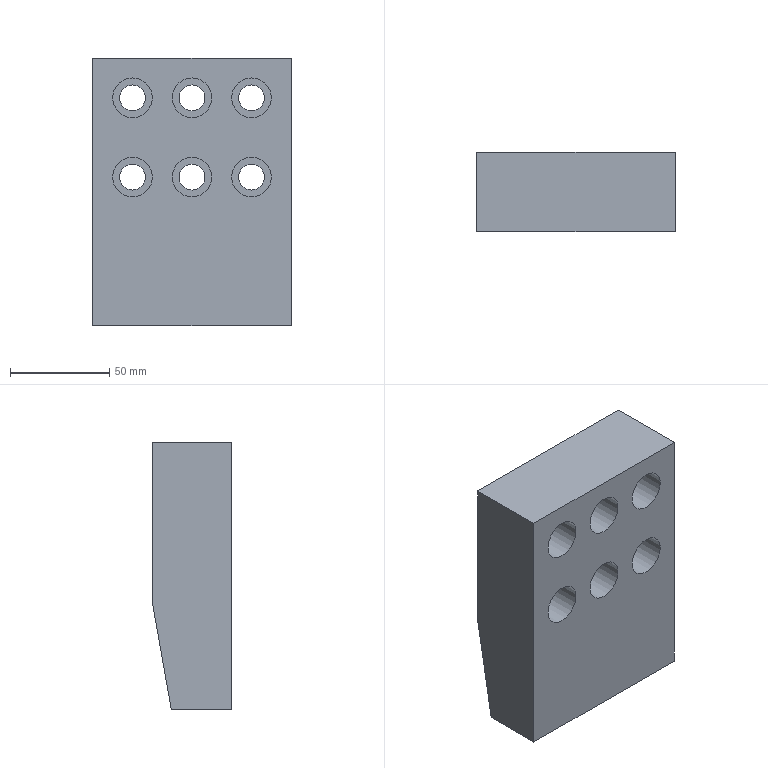Part | NX | features solid 2 | 1 solid | 25 faces | box 100 x 40 x 135 mm | volume 460372 mm3 | plane 13 | cylinder 12 | commonest cylinder face diameters 13 x6 20 x6
STEP:
#1=CARTESIAN_POINT('',(591.5,-905.,93.5));
#2=VERTEX_POINT('',#1);
#3=CARTESIAN_POINT('',(591.5,-905.,100.));
#4=DIRECTION('',(0.,1.,0.));
#5=DIRECTION('',(0.,0.,-1.));
#6=AXIS2_PLACEMENT_3D('',#3,#4,#5);
#7=CIRCLE('',#6,6.5);
#8=EDGE_CURVE('',#2,#2,#7,.T.);
#9=ORIENTED_EDGE('',*,*,#8,.F.);
#10=EDGE_LOOP('',(#9));
#11=FACE_BOUND('',#10,.T.);
#12=CARTESIAN_POINT('',(531.5,-905.,93.5));
#13=VERTEX_POINT('',#12);
#14=CARTESIAN_POINT('',(531.5,-905.,100.));
#15=DIRECTION('',(0.,1.,0.));
#16=DIRECTION('',(0.,0.,-1.));
#17=AXIS2_PLACEMENT_3D('',#14,#15,#16);
#18=CIRCLE('',#17,6.5);
#19=EDGE_CURVE('',#13,#13,#18,.T.);
#20=ORIENTED_EDGE('',*,*,#19,.F.);
#21=EDGE_LOOP('',(#20));
#22=FACE_BOUND('',#21,.T.);
#23=CARTESIAN_POINT('',(591.5,-905.,133.5));
#24=VERTEX_POINT('',#23);
#25=CARTESIAN_POINT('',(591.5,-905.,140.));
#26=DIRECTION('',(0.,1.,0.));
#27=DIRECTION('',(0.,0.,-1.));
#28=AXIS2_PLACEMENT_3D('',#25,#26,#27);
#29=CIRCLE('',#28,6.5);
#30=EDGE_CURVE('',#24,#24,#29,.T.);
#31=ORIENTED_EDGE('',*,*,#30,.F.);
#32=EDGE_LOOP('',(#31));
#33=FACE_BOUND('',#32,.T.);
#34=CARTESIAN_POINT('',(531.5,-905.,133.5));
#35=VERTEX_POINT('',#34);
#36=CARTESIAN_POINT('',(531.5,-905.,140.));
#37=DIRECTION('',(0.,1.,0.));
#38=DIRECTION('',(0.,0.,-1.));
#39=AXIS2_PLACEMENT_3D('',#36,#37,#38);
#40=CIRCLE('',#39,6.5);
#41=EDGE_CURVE('',#35,#35,#40,.T.);
#42=ORIENTED_EDGE('',*,*,#41,.F.);
#43=EDGE_LOOP('',(#42));
#44=FACE_BOUND('',#43,.T.);
#45=CARTESIAN_POINT('',(561.5,-905.,133.5));
#46=VERTEX_POINT('',#45);
#47=CARTESIAN_POINT('',(561.5,-905.,140.));
#48=DIRECTION('',(0.,1.,0.));
#49=DIRECTION('',(0.,0.,-1.));
#50=AXIS2_PLACEMENT_3D('',#47,#48,#49);
#51=CIRCLE('',#50,6.5);
#52=EDGE_CURVE('',#46,#46,#51,.T.);
#53=ORIENTED_EDGE('',*,*,#52,.F.);
#54=EDGE_LOOP('',(#53));
#55=FACE_BOUND('',#54,.T.);
#56=CARTESIAN_POINT('',(561.5,-905.,93.5));
#57=VERTEX_POINT('',#56);
#58=CARTESIAN_POINT('',(561.5,-905.,100.));
#59=DIRECTION('',(0.,1.,0.));
#60=DIRECTION('',(0.,0.,-1.));
#61=AXIS2_PLACEMENT_3D('',#58,#59,#60);
#62=CIRCLE('',#61,6.5);
#63=EDGE_CURVE('',#57,#57,#62,.T.);
#64=ORIENTED_EDGE('',*,*,#63,.F.);
#65=EDGE_LOOP('',(#64));
#66=FACE_BOUND('',#65,.T.);
#67=CARTESIAN_POINT('',(611.5,-905.,160.));
#68=VERTEX_POINT('',#67);
#69=CARTESIAN_POINT('',(611.5,-905.,79.306));
#70=VERTEX_POINT('',#69);
#71=CARTESIAN_POINT('',(611.5,-905.,160.));
#72=DIRECTION('',(0.,0.,-1.));
#73=VECTOR('',#72,1000.);
#74=LINE('',#71,#73);
#75=EDGE_CURVE('',#68,#70,#74,.T.);
#76=ORIENTED_EDGE('',*,*,#75,.T.);
#77=CARTESIAN_POINT('',(511.5,-905.,79.306));
#78=VERTEX_POINT('',#77);
#79=CARTESIAN_POINT('',(536.5,-905.,79.306));
#80=DIRECTION('',(-1.,0.,0.));
#81=VECTOR('',#80,1000.);
#82=LINE('',#79,#81);
#83=EDGE_CURVE('',#78,#70,#82,.F.);
#84=ORIENTED_EDGE('',*,*,#83,.F.);
#85=CARTESIAN_POINT('',(511.5,-905.,160.));
#86=VERTEX_POINT('',#85);
#87=CARTESIAN_POINT('',(511.5,-905.,75.));
#88=DIRECTION('',(0.,0.,1.));
#89=VECTOR('',#88,1000.);
#90=LINE('',#87,#89);
#91=EDGE_CURVE('',#78,#86,#90,.T.);
#92=ORIENTED_EDGE('',*,*,#91,.T.);
#93=CARTESIAN_POINT('',(551.5,-905.,160.));
#94=DIRECTION('',(1.,0.,0.));
#95=VECTOR('',#94,1000.);
#96=LINE('',#93,#95);
#97=EDGE_CURVE('',#86,#68,#96,.T.);
#98=ORIENTED_EDGE('',*,*,#97,.T.);
#99=EDGE_LOOP('',(#76,#84,#92,#98));
#100=FACE_BOUND('',#99,.T.);
#101=CARTESIAN_POINT('',(631.5,-905.,75.));
#102=DIRECTION('',(0.,1.,0.));
#103=DIRECTION('',(0.,0.,-1.));
#104=AXIS2_PLACEMENT_3D('',#101,#102,#103);
#105=PLANE('',#104);
#106=ADVANCED_FACE('',(#11,#22,#33,#44,#55,#66,#100),#105,.T.);
#107=ORIENTED_EDGE('',*,*,#75,.F.);
#108=CARTESIAN_POINT('',(611.5,-945.,160.));
#109=VERTEX_POINT('',#108);
#110=CARTESIAN_POINT('',(611.5,-945.,160.));
#111=DIRECTION('',(0.,1.,0.));
#112=VECTOR('',#111,1000.);
#113=LINE('',#110,#112);
#114=EDGE_CURVE('',#109,#68,#113,.T.);
#115=ORIENTED_EDGE('',*,*,#114,.F.);
#116=CARTESIAN_POINT('',(611.5,-945.,25.));
#117=VERTEX_POINT('',#116);
#118=CARTESIAN_POINT('',(611.5,-945.,160.));
#119=DIRECTION('',(0.,0.,-1.));
#120=VECTOR('',#119,1000.);
#121=LINE('',#118,#120);
#122=EDGE_CURVE('',#109,#117,#121,.T.);
#123=ORIENTED_EDGE('',*,*,#122,.T.);
#124=CARTESIAN_POINT('',(611.5,-914.576,25.));
#125=VERTEX_POINT('',#124);
#126=CARTESIAN_POINT('',(611.5,-340.,25.));
#127=DIRECTION('',(0.,1.,0.));
#128=VECTOR('',#127,1000.);
#129=LINE('',#126,#128);
#130=EDGE_CURVE('',#117,#125,#129,.T.);
#131=ORIENTED_EDGE('',*,*,#130,.T.);
#132=CARTESIAN_POINT('',(611.5,-892.407,150.726));
#133=DIRECTION('',(0.,-0.1736,-0.9848));
#134=VECTOR('',#133,1000.);
#135=LINE('',#132,#134);
#136=EDGE_CURVE('',#125,#70,#135,.F.);
#137=ORIENTED_EDGE('',*,*,#136,.T.);
#138=EDGE_LOOP('',(#107,#115,#123,#131,#137));
#139=FACE_BOUND('',#138,.T.);
#140=CARTESIAN_POINT('',(611.5,-945.,160.));
#141=DIRECTION('',(1.,0.,0.));
#142=DIRECTION('',(0.,0.,1.));
#143=AXIS2_PLACEMENT_3D('',#140,#141,#142);
#144=PLANE('',#143);
#145=ADVANCED_FACE('',(#139),#144,.T.);
#146=CARTESIAN_POINT('',(511.5,-945.,25.));
#147=VERTEX_POINT('',#146);
#148=CARTESIAN_POINT('',(511.5,-914.576,25.));
#149=VERTEX_POINT('',#148);
#150=CARTESIAN_POINT('',(511.5,-945.,25.));
#151=DIRECTION('',(0.,1.,0.));
#152=VECTOR('',#151,1000.);
#153=LINE('',#150,#152);
#154=EDGE_CURVE('',#147,#149,#153,.T.);
#155=ORIENTED_EDGE('',*,*,#154,.T.);
#156=CARTESIAN_POINT('',(536.5,-914.576,25.));
#157=DIRECTION('',(1.,0.,0.));
#158=VECTOR('',#157,1000.);
#159=LINE('',#156,#158);
#160=EDGE_CURVE('',#125,#149,#159,.F.);
#161=ORIENTED_EDGE('',*,*,#160,.F.);
#162=ORIENTED_EDGE('',*,*,#130,.F.);
#163=CARTESIAN_POINT('',(956.5,-945.,25.));
#164=DIRECTION('',(-1.,0.,0.));
#165=VECTOR('',#164,1000.);
#166=LINE('',#163,#165);
#167=EDGE_CURVE('',#117,#147,#166,.T.);
#168=ORIENTED_EDGE('',*,*,#167,.T.);
#169=EDGE_LOOP('',(#155,#161,#162,#168));
#170=FACE_BOUND('',#169,.T.);
#171=CARTESIAN_POINT('',(956.5,-340.,25.));
#172=DIRECTION('',(0.,0.,-1.));
#173=DIRECTION('',(1.,0.,0.));
#174=AXIS2_PLACEMENT_3D('',#171,#172,#173);
#175=PLANE('',#174);
#176=ADVANCED_FACE('',(#170),#175,.T.);
#177=ORIENTED_EDGE('',*,*,#91,.F.);
#178=CARTESIAN_POINT('',(511.5,-911.133,44.524));
#179=DIRECTION('',(0.,-0.1736,-0.9848));
#180=VECTOR('',#179,1000.);
#181=LINE('',#178,#180);
#182=EDGE_CURVE('',#149,#78,#181,.F.);
#183=ORIENTED_EDGE('',*,*,#182,.F.);
#184=ORIENTED_EDGE('',*,*,#154,.F.);
#185=CARTESIAN_POINT('',(511.5,-945.,160.));
#186=VERTEX_POINT('',#185);
#187=CARTESIAN_POINT('',(511.5,-945.,75.));
#188=DIRECTION('',(0.,0.,1.));
#189=VECTOR('',#188,1000.);
#190=LINE('',#187,#189);
#191=EDGE_CURVE('',#147,#186,#190,.T.);
#192=ORIENTED_EDGE('',*,*,#191,.T.);
#193=CARTESIAN_POINT('',(511.5,-945.,160.));
#194=DIRECTION('',(0.,1.,0.));
#195=VECTOR('',#194,1000.);
#196=LINE('',#193,#195);
#197=EDGE_CURVE('',#186,#86,#196,.T.);
#198=ORIENTED_EDGE('',*,*,#197,.T.);
#199=EDGE_LOOP('',(#177,#183,#184,#192,#198));
#200=FACE_BOUND('',#199,.T.);
#201=CARTESIAN_POINT('',(511.5,-945.,75.));
#202=DIRECTION('',(-1.,0.,0.));
#203=DIRECTION('',(0.,0.,-1.));
#204=AXIS2_PLACEMENT_3D('',#201,#202,#203);
#205=PLANE('',#204);
#206=ADVANCED_FACE('',(#200),#205,.T.);
#207=ORIENTED_EDGE('',*,*,#97,.F.);
#208=ORIENTED_EDGE('',*,*,#197,.F.);
#209=CARTESIAN_POINT('',(551.5,-945.,160.));
#210=DIRECTION('',(1.,0.,0.));
#211=VECTOR('',#210,1000.);
#212=LINE('',#209,#211);
#213=EDGE_CURVE('',#186,#109,#212,.T.);
#214=ORIENTED_EDGE('',*,*,#213,.T.);
#215=ORIENTED_EDGE('',*,*,#114,.T.);
#216=EDGE_LOOP('',(#207,#208,#214,#215));
#217=FACE_BOUND('',#216,.T.);
#218=CARTESIAN_POINT('',(551.5,-945.,160.));
#219=DIRECTION('',(0.,0.,1.));
#220=DIRECTION('',(-1.,0.,0.));
#221=AXIS2_PLACEMENT_3D('',#218,#219,#220);
#222=PLANE('',#221);
#223=ADVANCED_FACE('',(#217),#222,.T.);
#224=CARTESIAN_POINT('',(561.5,-945.,90.));
#225=VERTEX_POINT('',#224);
#226=CARTESIAN_POINT('',(561.5,-945.,100.));
#227=DIRECTION('',(0.,1.,0.));
#228=DIRECTION('',(0.,0.,-1.));
#229=AXIS2_PLACEMENT_3D('',#226,#227,#228);
#230=CIRCLE('',#229,10.);
#231=EDGE_CURVE('',#225,#225,#230,.T.);
#232=ORIENTED_EDGE('',*,*,#231,.T.);
#233=EDGE_LOOP('',(#232));
#234=FACE_BOUND('',#233,.T.);
#235=CARTESIAN_POINT('',(561.5,-945.,130.));
#236=VERTEX_POINT('',#235);
#237=CARTESIAN_POINT('',(561.5,-945.,140.));
#238=DIRECTION('',(0.,1.,0.));
#239=DIRECTION('',(0.,0.,-1.));
#240=AXIS2_PLACEMENT_3D('',#237,#238,#239);
#241=CIRCLE('',#240,10.);
#242=EDGE_CURVE('',#236,#236,#241,.T.);
#243=ORIENTED_EDGE('',*,*,#242,.T.);
#244=EDGE_LOOP('',(#243));
#245=FACE_BOUND('',#244,.T.);
#246=CARTESIAN_POINT('',(531.5,-945.,130.));
#247=VERTEX_POINT('',#246);
#248=CARTESIAN_POINT('',(531.5,-945.,140.));
#249=DIRECTION('',(0.,1.,0.));
#250=DIRECTION('',(0.,0.,-1.));
#251=AXIS2_PLACEMENT_3D('',#248,#249,#250);
#252=CIRCLE('',#251,10.);
#253=EDGE_CURVE('',#247,#247,#252,.T.);
#254=ORIENTED_EDGE('',*,*,#253,.T.);
#255=EDGE_LOOP('',(#254));
#256=FACE_BOUND('',#255,.T.);
#257=CARTESIAN_POINT('',(591.5,-945.,130.));
#258=VERTEX_POINT('',#257);
#259=CARTESIAN_POINT('',(591.5,-945.,140.));
#260=DIRECTION('',(0.,1.,0.));
#261=DIRECTION('',(0.,0.,-1.));
#262=AXIS2_PLACEMENT_3D('',#259,#260,#261);
#263=CIRCLE('',#262,10.);
#264=EDGE_CURVE('',#258,#258,#263,.T.);
#265=ORIENTED_EDGE('',*,*,#264,.T.);
#266=EDGE_LOOP('',(#265));
#267=FACE_BOUND('',#266,.T.);
#268=CARTESIAN_POINT('',(531.5,-945.,90.));
#269=VERTEX_POINT('',#268);
#270=CARTESIAN_POINT('',(531.5,-945.,100.));
#271=DIRECTION('',(0.,1.,0.));
#272=DIRECTION('',(0.,0.,-1.));
#273=AXIS2_PLACEMENT_3D('',#270,#271,#272);
#274=CIRCLE('',#273,10.);
#275=EDGE_CURVE('',#269,#269,#274,.T.);
#276=ORIENTED_EDGE('',*,*,#275,.T.);
#277=EDGE_LOOP('',(#276));
#278=FACE_BOUND('',#277,.T.);
#279=CARTESIAN_POINT('',(591.5,-945.,90.));
#280=VERTEX_POINT('',#279);
#281=CARTESIAN_POINT('',(591.5,-945.,100.));
#282=DIRECTION('',(0.,1.,0.));
#283=DIRECTION('',(0.,0.,-1.));
#284=AXIS2_PLACEMENT_3D('',#281,#282,#283);
#285=CIRCLE('',#284,10.);
#286=EDGE_CURVE('',#280,#280,#285,.T.);
#287=ORIENTED_EDGE('',*,*,#286,.T.);
#288=EDGE_LOOP('',(#287));
#289=FACE_BOUND('',#288,.T.);
#290=ORIENTED_EDGE('',*,*,#122,.F.);
#291=ORIENTED_EDGE('',*,*,#213,.F.);
#292=ORIENTED_EDGE('',*,*,#191,.F.);
#293=ORIENTED_EDGE('',*,*,#167,.F.);
#294=EDGE_LOOP('',(#290,#291,#292,#293));
#295=FACE_BOUND('',#294,.T.);
#296=CARTESIAN_POINT('',(631.5,-945.,75.));
#297=DIRECTION('',(0.,1.,0.));
#298=DIRECTION('',(0.,0.,-1.));
#299=AXIS2_PLACEMENT_3D('',#296,#297,#298);
#300=PLANE('',#299);
#301=ADVANCED_FACE('',(#234,#245,#256,#267,#278,#289,#295),#300,.F.);
#302=ORIENTED_EDGE('',*,*,#8,.T.);
#303=EDGE_LOOP('',(#302));
#304=FACE_BOUND('',#303,.T.);
#305=CARTESIAN_POINT('',(591.5,-925.,93.5));
#306=VERTEX_POINT('',#305);
#307=CARTESIAN_POINT('',(591.5,-925.,100.));
#308=DIRECTION('',(0.,1.,0.));
#309=DIRECTION('',(0.,0.,-1.));
#310=AXIS2_PLACEMENT_3D('',#307,#308,#309);
#311=CIRCLE('',#310,6.5);
#312=EDGE_CURVE('',#306,#306,#311,.T.);
#313=ORIENTED_EDGE('',*,*,#312,.F.);
#314=EDGE_LOOP('',(#313));
#315=FACE_BOUND('',#314,.T.);
#316=CARTESIAN_POINT('',(591.5,-895.,100.));
#317=DIRECTION('',(0.,1.,0.));
#318=DIRECTION('',(0.,0.,-1.));
#319=AXIS2_PLACEMENT_3D('',#316,#317,#318);
#320=CYLINDRICAL_SURFACE('',#319,6.5);
#321=ADVANCED_FACE('',(#304,#315),#320,.F.);
#322=ORIENTED_EDGE('',*,*,#312,.T.);
#323=EDGE_LOOP('',(#322));
#324=FACE_BOUND('',#323,.T.);
#325=CARTESIAN_POINT('',(591.5,-925.,90.));
#326=VERTEX_POINT('',#325);
#327=CARTESIAN_POINT('',(591.5,-925.,100.));
#328=DIRECTION('',(0.,1.,0.));
#329=DIRECTION('',(0.,0.,-1.));
#330=AXIS2_PLACEMENT_3D('',#327,#328,#329);
#331=CIRCLE('',#330,10.);
#332=EDGE_CURVE('',#326,#326,#331,.T.);
#333=ORIENTED_EDGE('',*,*,#332,.F.);
#334=EDGE_LOOP('',(#333));
#335=FACE_BOUND('',#334,.T.);
#336=CARTESIAN_POINT('',(611.5,-925.,100.));
#337=DIRECTION('',(0.,1.,0.));
#338=DIRECTION('',(0.,0.,-1.));
#339=AXIS2_PLACEMENT_3D('',#336,#337,#338);
#340=PLANE('',#339);
#341=ADVANCED_FACE('',(#324,#335),#340,.F.);
#342=ORIENTED_EDGE('',*,*,#332,.T.);
#343=EDGE_LOOP('',(#342));
#344=FACE_BOUND('',#343,.T.);
#345=ORIENTED_EDGE('',*,*,#286,.F.);
#346=EDGE_LOOP('',(#345));
#347=FACE_BOUND('',#346,.T.);
#348=CARTESIAN_POINT('',(591.5,-945.,100.));
#349=DIRECTION('',(0.,1.,0.));
#350=DIRECTION('',(0.,0.,-1.));
#351=AXIS2_PLACEMENT_3D('',#348,#349,#350);
#352=CYLINDRICAL_SURFACE('',#351,10.);
#353=ADVANCED_FACE('',(#344,#347),#352,.F.);
#354=ORIENTED_EDGE('',*,*,#19,.T.);
#355=EDGE_LOOP('',(#354));
#356=FACE_BOUND('',#355,.T.);
#357=CARTESIAN_POINT('',(531.5,-925.,93.5));
#358=VERTEX_POINT('',#357);
#359=CARTESIAN_POINT('',(531.5,-925.,100.));
#360=DIRECTION('',(0.,1.,0.));
#361=DIRECTION('',(0.,0.,-1.));
#362=AXIS2_PLACEMENT_3D('',#359,#360,#361);
#363=CIRCLE('',#362,6.5);
#364=EDGE_CURVE('',#358,#358,#363,.T.);
#365=ORIENTED_EDGE('',*,*,#364,.F.);
#366=EDGE_LOOP('',(#365));
#367=FACE_BOUND('',#366,.T.);
#368=CARTESIAN_POINT('',(531.5,-895.,100.));
#369=DIRECTION('',(0.,1.,0.));
#370=DIRECTION('',(0.,0.,-1.));
#371=AXIS2_PLACEMENT_3D('',#368,#369,#370);
#372=CYLINDRICAL_SURFACE('',#371,6.5);
#373=ADVANCED_FACE('',(#356,#367),#372,.F.);
#374=ORIENTED_EDGE('',*,*,#364,.T.);
#375=EDGE_LOOP('',(#374));
#376=FACE_BOUND('',#375,.T.);
#377=CARTESIAN_POINT('',(531.5,-925.,90.));
#378=VERTEX_POINT('',#377);
#379=CARTESIAN_POINT('',(531.5,-925.,100.));
#380=DIRECTION('',(0.,1.,0.));
#381=DIRECTION('',(0.,0.,-1.));
#382=AXIS2_PLACEMENT_3D('',#379,#380,#381);
#383=CIRCLE('',#382,10.);
#384=EDGE_CURVE('',#378,#378,#383,.T.);
#385=ORIENTED_EDGE('',*,*,#384,.F.);
#386=EDGE_LOOP('',(#385));
#387=FACE_BOUND('',#386,.T.);
#388=CARTESIAN_POINT('',(531.5,-925.,100.));
#389=DIRECTION('',(0.,1.,0.));
#390=DIRECTION('',(0.,0.,-1.));
#391=AXIS2_PLACEMENT_3D('',#388,#389,#390);
#392=PLANE('',#391);
#393=ADVANCED_FACE('',(#376,#387),#392,.F.);
#394=ORIENTED_EDGE('',*,*,#384,.T.);
#395=EDGE_LOOP('',(#394));
#396=FACE_BOUND('',#395,.T.);
#397=ORIENTED_EDGE('',*,*,#275,.F.);
#398=EDGE_LOOP('',(#397));
#399=FACE_BOUND('',#398,.T.);
#400=CARTESIAN_POINT('',(531.5,-945.,100.));
#401=DIRECTION('',(0.,1.,0.));
#402=DIRECTION('',(0.,0.,-1.));
#403=AXIS2_PLACEMENT_3D('',#400,#401,#402);
#404=CYLINDRICAL_SURFACE('',#403,10.);
#405=ADVANCED_FACE('',(#396,#399),#404,.F.);
#406=ORIENTED_EDGE('',*,*,#30,.T.);
#407=EDGE_LOOP('',(#406));
#408=FACE_BOUND('',#407,.T.);
#409=CARTESIAN_POINT('',(591.5,-925.,133.5));
#410=VERTEX_POINT('',#409);
#411=CARTESIAN_POINT('',(591.5,-925.,140.));
#412=DIRECTION('',(0.,1.,0.));
#413=DIRECTION('',(0.,0.,-1.));
#414=AXIS2_PLACEMENT_3D('',#411,#412,#413);
#415=CIRCLE('',#414,6.5);
#416=EDGE_CURVE('',#410,#410,#415,.T.);
#417=ORIENTED_EDGE('',*,*,#416,.F.);
#418=EDGE_LOOP('',(#417));
#419=FACE_BOUND('',#418,.T.);
#420=CARTESIAN_POINT('',(591.5,-895.,140.));
#421=DIRECTION('',(0.,1.,0.));
#422=DIRECTION('',(0.,0.,-1.));
#423=AXIS2_PLACEMENT_3D('',#420,#421,#422);
#424=CYLINDRICAL_SURFACE('',#423,6.5);
#425=ADVANCED_FACE('',(#408,#419),#424,.F.);
#426=ORIENTED_EDGE('',*,*,#416,.T.);
#427=EDGE_LOOP('',(#426));
#428=FACE_BOUND('',#427,.T.);
#429=CARTESIAN_POINT('',(591.5,-925.,130.));
#430=VERTEX_POINT('',#429);
#431=CARTESIAN_POINT('',(591.5,-925.,140.));
#432=DIRECTION('',(0.,1.,0.));
#433=DIRECTION('',(0.,0.,-1.));
#434=AXIS2_PLACEMENT_3D('',#431,#432,#433);
#435=CIRCLE('',#434,10.);
#436=EDGE_CURVE('',#430,#430,#435,.T.);
#437=ORIENTED_EDGE('',*,*,#436,.F.);
#438=EDGE_LOOP('',(#437));
#439=FACE_BOUND('',#438,.T.);
#440=CARTESIAN_POINT('',(611.5,-925.,140.));
#441=DIRECTION('',(0.,1.,0.));
#442=DIRECTION('',(0.,0.,-1.));
#443=AXIS2_PLACEMENT_3D('',#440,#441,#442);
#444=PLANE('',#443);
#445=ADVANCED_FACE('',(#428,#439),#444,.F.);
#446=ORIENTED_EDGE('',*,*,#436,.T.);
#447=EDGE_LOOP('',(#446));
#448=FACE_BOUND('',#447,.T.);
#449=ORIENTED_EDGE('',*,*,#264,.F.);
#450=EDGE_LOOP('',(#449));
#451=FACE_BOUND('',#450,.T.);
#452=CARTESIAN_POINT('',(591.5,-945.,140.));
#453=DIRECTION('',(0.,1.,0.));
#454=DIRECTION('',(0.,0.,-1.));
#455=AXIS2_PLACEMENT_3D('',#452,#453,#454);
#456=CYLINDRICAL_SURFACE('',#455,10.);
#457=ADVANCED_FACE('',(#448,#451),#456,.F.);
#458=ORIENTED_EDGE('',*,*,#41,.T.);
#459=EDGE_LOOP('',(#458));
#460=FACE_BOUND('',#459,.T.);
#461=CARTESIAN_POINT('',(531.5,-925.,133.5));
#462=VERTEX_POINT('',#461);
#463=CARTESIAN_POINT('',(531.5,-925.,140.));
#464=DIRECTION('',(0.,1.,0.));
#465=DIRECTION('',(0.,0.,-1.));
#466=AXIS2_PLACEMENT_3D('',#463,#464,#465);
#467=CIRCLE('',#466,6.5);
#468=EDGE_CURVE('',#462,#462,#467,.T.);
#469=ORIENTED_EDGE('',*,*,#468,.F.);
#470=EDGE_LOOP('',(#469));
#471=FACE_BOUND('',#470,.T.);
#472=CARTESIAN_POINT('',(531.5,-895.,140.));
#473=DIRECTION('',(0.,1.,0.));
#474=DIRECTION('',(0.,0.,-1.));
#475=AXIS2_PLACEMENT_3D('',#472,#473,#474);
#476=CYLINDRICAL_SURFACE('',#475,6.5);
#477=ADVANCED_FACE('',(#460,#471),#476,.F.);
#478=ORIENTED_EDGE('',*,*,#468,.T.);
#479=EDGE_LOOP('',(#478));
#480=FACE_BOUND('',#479,.T.);
#481=CARTESIAN_POINT('',(531.5,-925.,130.));
#482=VERTEX_POINT('',#481);
#483=CARTESIAN_POINT('',(531.5,-925.,140.));
#484=DIRECTION('',(0.,1.,0.));
#485=DIRECTION('',(0.,0.,-1.));
#486=AXIS2_PLACEMENT_3D('',#483,#484,#485);
#487=CIRCLE('',#486,10.);
#488=EDGE_CURVE('',#482,#482,#487,.T.);
#489=ORIENTED_EDGE('',*,*,#488,.F.);
#490=EDGE_LOOP('',(#489));
#491=FACE_BOUND('',#490,.T.);
#492=CARTESIAN_POINT('',(531.5,-925.,140.));
#493=DIRECTION('',(0.,1.,0.));
#494=DIRECTION('',(0.,0.,-1.));
#495=AXIS2_PLACEMENT_3D('',#492,#493,#494);
#496=PLANE('',#495);
#497=ADVANCED_FACE('',(#480,#491),#496,.F.);
#498=ORIENTED_EDGE('',*,*,#488,.T.);
#499=EDGE_LOOP('',(#498));
#500=FACE_BOUND('',#499,.T.);
#501=ORIENTED_EDGE('',*,*,#253,.F.);
#502=EDGE_LOOP('',(#501));
#503=FACE_BOUND('',#502,.T.);
#504=CARTESIAN_POINT('',(531.5,-945.,140.));
#505=DIRECTION('',(0.,1.,0.));
#506=DIRECTION('',(0.,0.,-1.));
#507=AXIS2_PLACEMENT_3D('',#504,#505,#506);
#508=CYLINDRICAL_SURFACE('',#507,10.);
#509=ADVANCED_FACE('',(#500,#503),#508,.F.);
#510=ORIENTED_EDGE('',*,*,#52,.T.);
#511=EDGE_LOOP('',(#510));
#512=FACE_BOUND('',#511,.T.);
#513=CARTESIAN_POINT('',(561.5,-925.,133.5));
#514=VERTEX_POINT('',#513);
#515=CARTESIAN_POINT('',(561.5,-925.,140.));
#516=DIRECTION('',(0.,1.,0.));
#517=DIRECTION('',(0.,0.,-1.));
#518=AXIS2_PLACEMENT_3D('',#515,#516,#517);
#519=CIRCLE('',#518,6.5);
#520=EDGE_CURVE('',#514,#514,#519,.T.);
#521=ORIENTED_EDGE('',*,*,#520,.F.);
#522=EDGE_LOOP('',(#521));
#523=FACE_BOUND('',#522,.T.);
#524=CARTESIAN_POINT('',(561.5,-895.,140.));
#525=DIRECTION('',(0.,1.,0.));
#526=DIRECTION('',(0.,0.,-1.));
#527=AXIS2_PLACEMENT_3D('',#524,#525,#526);
#528=CYLINDRICAL_SURFACE('',#527,6.5);
#529=ADVANCED_FACE('',(#512,#523),#528,.F.);
#530=ORIENTED_EDGE('',*,*,#520,.T.);
#531=EDGE_LOOP('',(#530));
#532=FACE_BOUND('',#531,.T.);
#533=CARTESIAN_POINT('',(561.5,-925.,130.));
#534=VERTEX_POINT('',#533);
#535=CARTESIAN_POINT('',(561.5,-925.,140.));
#536=DIRECTION('',(0.,1.,0.));
#537=DIRECTION('',(0.,0.,-1.));
#538=AXIS2_PLACEMENT_3D('',#535,#536,#537);
#539=CIRCLE('',#538,10.);
#540=EDGE_CURVE('',#534,#534,#539,.T.);
#541=ORIENTED_EDGE('',*,*,#540,.F.);
#542=EDGE_LOOP('',(#541));
#543=FACE_BOUND('',#542,.T.);
#544=CARTESIAN_POINT('',(561.5,-925.,140.));
#545=DIRECTION('',(0.,1.,0.));
#546=DIRECTION('',(0.,0.,-1.));
#547=AXIS2_PLACEMENT_3D('',#544,#545,#546);
#548=PLANE('',#547);
#549=ADVANCED_FACE('',(#532,#543),#548,.F.);
#550=ORIENTED_EDGE('',*,*,#540,.T.);
#551=EDGE_LOOP('',(#550));
#552=FACE_BOUND('',#551,.T.);
#553=ORIENTED_EDGE('',*,*,#242,.F.);
#554=EDGE_LOOP('',(#553));
#555=FACE_BOUND('',#554,.T.);
#556=CARTESIAN_POINT('',(561.5,-945.,140.));
#557=DIRECTION('',(0.,1.,0.));
#558=DIRECTION('',(0.,0.,-1.));
#559=AXIS2_PLACEMENT_3D('',#556,#557,#558);
#560=CYLINDRICAL_SURFACE('',#559,10.);
#561=ADVANCED_FACE('',(#552,#555),#560,.F.);
#562=ORIENTED_EDGE('',*,*,#63,.T.);
#563=EDGE_LOOP('',(#562));
#564=FACE_BOUND('',#563,.T.);
#565=CARTESIAN_POINT('',(561.5,-925.,93.5));
#566=VERTEX_POINT('',#565);
#567=CARTESIAN_POINT('',(561.5,-925.,100.));
#568=DIRECTION('',(0.,1.,0.));
#569=DIRECTION('',(0.,0.,-1.));
#570=AXIS2_PLACEMENT_3D('',#567,#568,#569);
#571=CIRCLE('',#570,6.5);
#572=EDGE_CURVE('',#566,#566,#571,.T.);
#573=ORIENTED_EDGE('',*,*,#572,.F.);
#574=EDGE_LOOP('',(#573));
#575=FACE_BOUND('',#574,.T.);
#576=CARTESIAN_POINT('',(561.5,-895.,100.));
#577=DIRECTION('',(0.,1.,0.));
#578=DIRECTION('',(0.,0.,-1.));
#579=AXIS2_PLACEMENT_3D('',#576,#577,#578);
#580=CYLINDRICAL_SURFACE('',#579,6.5);
#581=ADVANCED_FACE('',(#564,#575),#580,.F.);
#582=ORIENTED_EDGE('',*,*,#572,.T.);
#583=EDGE_LOOP('',(#582));
#584=FACE_BOUND('',#583,.T.);
#585=CARTESIAN_POINT('',(561.5,-925.,90.));
#586=VERTEX_POINT('',#585);
#587=CARTESIAN_POINT('',(561.5,-925.,100.));
#588=DIRECTION('',(0.,1.,0.));
#589=DIRECTION('',(0.,0.,-1.));
#590=AXIS2_PLACEMENT_3D('',#587,#588,#589);
#591=CIRCLE('',#590,10.);
#592=EDGE_CURVE('',#586,#586,#591,.T.);
#593=ORIENTED_EDGE('',*,*,#592,.F.);
#594=EDGE_LOOP('',(#593));
#595=FACE_BOUND('',#594,.T.);
#596=CARTESIAN_POINT('',(561.5,-925.,100.));
#597=DIRECTION('',(0.,1.,0.));
#598=DIRECTION('',(0.,0.,-1.));
#599=AXIS2_PLACEMENT_3D('',#596,#597,#598);
#600=PLANE('',#599);
#601=ADVANCED_FACE('',(#584,#595),#600,.F.);
#602=ORIENTED_EDGE('',*,*,#592,.T.);
#603=EDGE_LOOP('',(#602));
#604=FACE_BOUND('',#603,.T.);
#605=ORIENTED_EDGE('',*,*,#231,.F.);
#606=EDGE_LOOP('',(#605));
#607=FACE_BOUND('',#606,.T.);
#608=CARTESIAN_POINT('',(561.5,-945.,100.));
#609=DIRECTION('',(0.,1.,0.));
#610=DIRECTION('',(0.,0.,-1.));
#611=AXIS2_PLACEMENT_3D('',#608,#609,#610);
#612=CYLINDRICAL_SURFACE('',#611,10.);
#613=ADVANCED_FACE('',(#604,#607),#612,.F.);
#614=ORIENTED_EDGE('',*,*,#182,.T.);
#615=ORIENTED_EDGE('',*,*,#83,.T.);
#616=ORIENTED_EDGE('',*,*,#136,.F.);
#617=ORIENTED_EDGE('',*,*,#160,.T.);
#618=EDGE_LOOP('',(#614,#615,#616,#617));
#619=FACE_BOUND('',#618,.T.);
#620=CARTESIAN_POINT('',(536.5,-911.133,44.524));
#621=DIRECTION('',(0.,0.9848,-0.1736));
#622=DIRECTION('',(0.,-0.1736,-0.9848));
#623=AXIS2_PLACEMENT_3D('',#620,#621,#622);
#624=PLANE('',#623);
#625=ADVANCED_FACE('',(#619),#624,.T.);
#626=CLOSED_SHELL('',(#106,#145,#176,#206,#223,#301,#321,#341,#353,#373,#393,#405,#425,#445,#457,#477,#497,#509,#529,#549,#561,#581,#601,#613,#625));
#627=MANIFOLD_SOLID_BREP('',#626);
#628=(LENGTH_UNIT()NAMED_UNIT(*)SI_UNIT(.MILLI.,.METRE.));
#629=UNCERTAINTY_MEASURE_WITH_UNIT(LENGTH_MEASURE(0.00001),#628,'','');
#630=(NAMED_UNIT(*)PLANE_ANGLE_UNIT()SI_UNIT($,.RADIAN.));
#631=(NAMED_UNIT(*)SI_UNIT($,.STERADIAN.)SOLID_ANGLE_UNIT());
#632=(GEOMETRIC_REPRESENTATION_CONTEXT(3)GLOBAL_UNCERTAINTY_ASSIGNED_CONTEXT((#629))GLOBAL_UNIT_ASSIGNED_CONTEXT((#628,#630,#631))REPRESENTATION_CONTEXT('',''));
#633=ADVANCED_BREP_SHAPE_REPRESENTATION('',(#627),#632);